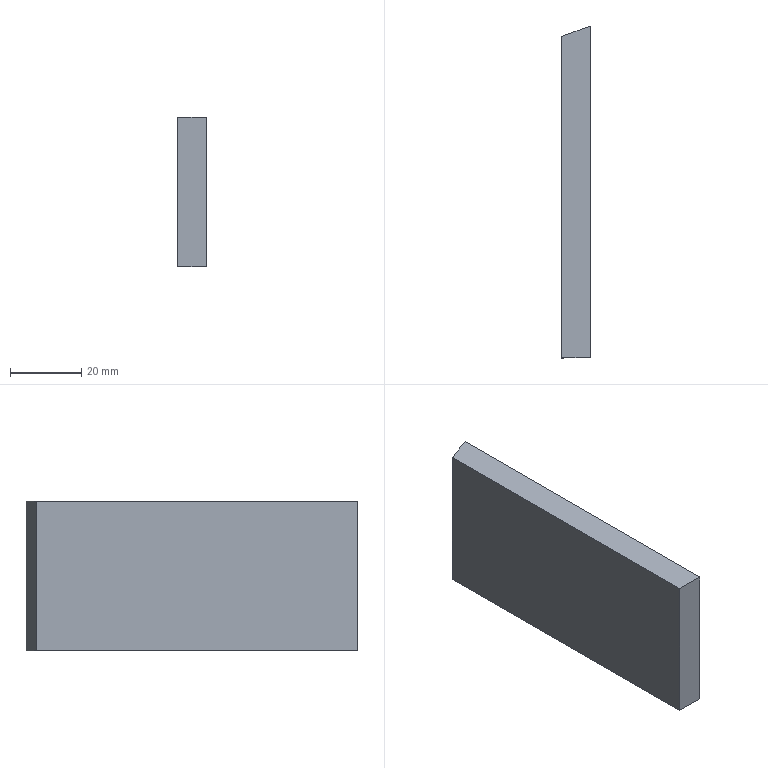Part | SolidWorks | features Extrusion 1, ICE 1 | 1 solid | 6 faces | box 8 x 93.358 x 42 mm | volume 30876 mm3 | plane 6
STEP:
#1=CARTESIAN_POINT('',(176.478,283.425,0.));
#2=VERTEX_POINT('',#1);
#3=CARTESIAN_POINT('',(176.478,193.,0.));
#4=VERTEX_POINT('',#3);
#5=CARTESIAN_POINT('',(176.478,283.425,0.));
#6=DIRECTION('',(0.,-1.,0.));
#7=VECTOR('',#6,1000.);
#8=LINE('',#5,#7);
#9=EDGE_CURVE('',#2,#4,#8,.T.);
#10=ORIENTED_EDGE('',*,*,#9,.T.);
#11=CARTESIAN_POINT('',(176.478,193.,42.));
#12=VERTEX_POINT('',#11);
#13=CARTESIAN_POINT('',(176.478,193.,25.));
#14=DIRECTION('',(0.,0.,-1.));
#15=VECTOR('',#14,1000.);
#16=LINE('',#13,#15);
#17=EDGE_CURVE('',#12,#4,#16,.T.);
#18=ORIENTED_EDGE('',*,*,#17,.F.);
#19=CARTESIAN_POINT('',(176.478,283.425,42.));
#20=VERTEX_POINT('',#19);
#21=CARTESIAN_POINT('',(176.478,283.425,42.));
#22=DIRECTION('',(0.,-1.,0.));
#23=VECTOR('',#22,1000.);
#24=LINE('',#21,#23);
#25=EDGE_CURVE('',#20,#12,#24,.T.);
#26=ORIENTED_EDGE('',*,*,#25,.F.);
#27=CARTESIAN_POINT('',(176.478,283.425,25.));
#28=DIRECTION('',(0.,0.,-1.));
#29=VECTOR('',#28,1000.);
#30=LINE('',#27,#29);
#31=EDGE_CURVE('',#20,#2,#30,.T.);
#32=ORIENTED_EDGE('',*,*,#31,.T.);
#33=EDGE_LOOP('',(#10,#18,#26,#32));
#34=FACE_OUTER_BOUND('',#33,.T.);
#35=CARTESIAN_POINT('',(176.478,283.425,25.));
#36=DIRECTION('',(1.,0.,0.));
#37=DIRECTION('',(0.,0.,-1.));
#38=AXIS2_PLACEMENT_3D('',#35,#36,#37);
#39=PLANE('',#38);
#40=ADVANCED_FACE('',(#34),#39,.F.);
#41=CARTESIAN_POINT('',(184.478,193.,0.));
#42=VERTEX_POINT('',#41);
#43=CARTESIAN_POINT('',(176.478,193.,0.));
#44=DIRECTION('',(1.,0.,0.));
#45=VECTOR('',#44,1000.);
#46=LINE('',#43,#45);
#47=EDGE_CURVE('',#4,#42,#46,.T.);
#48=ORIENTED_EDGE('',*,*,#47,.T.);
#49=CARTESIAN_POINT('',(184.478,193.,42.));
#50=VERTEX_POINT('',#49);
#51=CARTESIAN_POINT('',(184.478,193.,25.));
#52=DIRECTION('',(0.,0.,-1.));
#53=VECTOR('',#52,1000.);
#54=LINE('',#51,#53);
#55=EDGE_CURVE('',#50,#42,#54,.T.);
#56=ORIENTED_EDGE('',*,*,#55,.F.);
#57=CARTESIAN_POINT('',(176.478,193.,42.));
#58=DIRECTION('',(1.,0.,0.));
#59=VECTOR('',#58,1000.);
#60=LINE('',#57,#59);
#61=EDGE_CURVE('',#12,#50,#60,.T.);
#62=ORIENTED_EDGE('',*,*,#61,.F.);
#63=ORIENTED_EDGE('',*,*,#17,.T.);
#64=EDGE_LOOP('',(#48,#56,#62,#63));
#65=FACE_OUTER_BOUND('',#64,.T.);
#66=CARTESIAN_POINT('',(176.478,193.,25.));
#67=DIRECTION('',(0.,1.,0.));
#68=DIRECTION('',(-1.,0.,0.));
#69=AXIS2_PLACEMENT_3D('',#66,#67,#68);
#70=PLANE('',#69);
#71=ADVANCED_FACE('',(#65),#70,.F.);
#72=CARTESIAN_POINT('',(184.478,286.358,0.));
#73=VERTEX_POINT('',#72);
#74=CARTESIAN_POINT('',(184.478,193.,0.));
#75=DIRECTION('',(0.,1.,0.));
#76=VECTOR('',#75,1000.);
#77=LINE('',#74,#76);
#78=EDGE_CURVE('',#42,#73,#77,.T.);
#79=ORIENTED_EDGE('',*,*,#78,.T.);
#80=CARTESIAN_POINT('',(184.478,286.358,42.));
#81=VERTEX_POINT('',#80);
#82=CARTESIAN_POINT('',(184.478,286.358,25.));
#83=DIRECTION('',(0.,0.,-1.));
#84=VECTOR('',#83,1000.);
#85=LINE('',#82,#84);
#86=EDGE_CURVE('',#81,#73,#85,.T.);
#87=ORIENTED_EDGE('',*,*,#86,.F.);
#88=CARTESIAN_POINT('',(184.478,193.,42.));
#89=DIRECTION('',(0.,1.,0.));
#90=VECTOR('',#89,1000.);
#91=LINE('',#88,#90);
#92=EDGE_CURVE('',#50,#81,#91,.T.);
#93=ORIENTED_EDGE('',*,*,#92,.F.);
#94=ORIENTED_EDGE('',*,*,#55,.T.);
#95=EDGE_LOOP('',(#79,#87,#93,#94));
#96=FACE_OUTER_BOUND('',#95,.T.);
#97=CARTESIAN_POINT('',(184.478,193.,25.));
#98=DIRECTION('',(-1.,0.,0.));
#99=DIRECTION('',(0.,-1.,0.));
#100=AXIS2_PLACEMENT_3D('',#97,#98,#99);
#101=PLANE('',#100);
#102=ADVANCED_FACE('',(#96),#101,.F.);
#103=CARTESIAN_POINT('',(184.478,286.358,0.));
#104=DIRECTION('',(-0.9389,-0.3443,0.));
#105=VECTOR('',#104,1000.);
#106=LINE('',#103,#105);
#107=EDGE_CURVE('',#73,#2,#106,.T.);
#108=ORIENTED_EDGE('',*,*,#107,.T.);
#109=ORIENTED_EDGE('',*,*,#31,.F.);
#110=CARTESIAN_POINT('',(184.478,286.358,42.));
#111=DIRECTION('',(-0.9389,-0.3443,0.));
#112=VECTOR('',#111,1000.);
#113=LINE('',#110,#112);
#114=EDGE_CURVE('',#81,#20,#113,.T.);
#115=ORIENTED_EDGE('',*,*,#114,.F.);
#116=ORIENTED_EDGE('',*,*,#86,.T.);
#117=EDGE_LOOP('',(#108,#109,#115,#116));
#118=FACE_OUTER_BOUND('',#117,.T.);
#119=CARTESIAN_POINT('',(184.478,286.358,25.));
#120=DIRECTION('',(0.3443,-0.9389,0.));
#121=DIRECTION('',(0.9389,0.3443,0.));
#122=AXIS2_PLACEMENT_3D('',#119,#120,#121);
#123=PLANE('',#122);
#124=ADVANCED_FACE('',(#118),#123,.F.);
#125=ORIENTED_EDGE('',*,*,#9,.F.);
#126=ORIENTED_EDGE('',*,*,#107,.F.);
#127=ORIENTED_EDGE('',*,*,#78,.F.);
#128=ORIENTED_EDGE('',*,*,#47,.F.);
#129=EDGE_LOOP('',(#125,#126,#127,#128));
#130=FACE_OUTER_BOUND('',#129,.T.);
#131=CARTESIAN_POINT('',(0.,0.,0.));
#132=DIRECTION('',(0.,0.,1.));
#133=DIRECTION('',(1.,0.,0.));
#134=AXIS2_PLACEMENT_3D('',#131,#132,#133);
#135=PLANE('',#134);
#136=ADVANCED_FACE('',(#130),#135,.F.);
#137=ORIENTED_EDGE('',*,*,#114,.T.);
#138=ORIENTED_EDGE('',*,*,#25,.T.);
#139=ORIENTED_EDGE('',*,*,#61,.T.);
#140=ORIENTED_EDGE('',*,*,#92,.T.);
#141=EDGE_LOOP('',(#137,#138,#139,#140));
#142=FACE_OUTER_BOUND('',#141,.T.);
#143=CARTESIAN_POINT('',(0.,0.,42.));
#144=DIRECTION('',(0.,0.,1.));
#145=DIRECTION('',(1.,0.,0.));
#146=AXIS2_PLACEMENT_3D('',#143,#144,#145);
#147=PLANE('',#146);
#148=ADVANCED_FACE('',(#142),#147,.T.);
#149=CLOSED_SHELL('',(#40,#71,#102,#124,#136,#148));
#150=MANIFOLD_SOLID_BREP('',#149);
#151=CARTESIAN_POINT('',(0.,0.,0.));
#152=DIRECTION('',(0.,0.,1.));
#153=DIRECTION('',(1.,0.,0.));
#154=AXIS2_PLACEMENT_3D('',#151,#152,#153);
#155=(LENGTH_UNIT()NAMED_UNIT(*)SI_UNIT(.MILLI.,.METRE.));
#156=UNCERTAINTY_MEASURE_WITH_UNIT(LENGTH_MEASURE(0.00001),#155,'','');
#157=(NAMED_UNIT(*)PLANE_ANGLE_UNIT()SI_UNIT($,.RADIAN.));
#158=(NAMED_UNIT(*)SI_UNIT($,.STERADIAN.)SOLID_ANGLE_UNIT());
#159=(GEOMETRIC_REPRESENTATION_CONTEXT(3)GLOBAL_UNCERTAINTY_ASSIGNED_CONTEXT((#156))GLOBAL_UNIT_ASSIGNED_CONTEXT((#155,#157,#158))REPRESENTATION_CONTEXT('',''));
#160=ADVANCED_BREP_SHAPE_REPRESENTATION('',(#150,#154),#159);